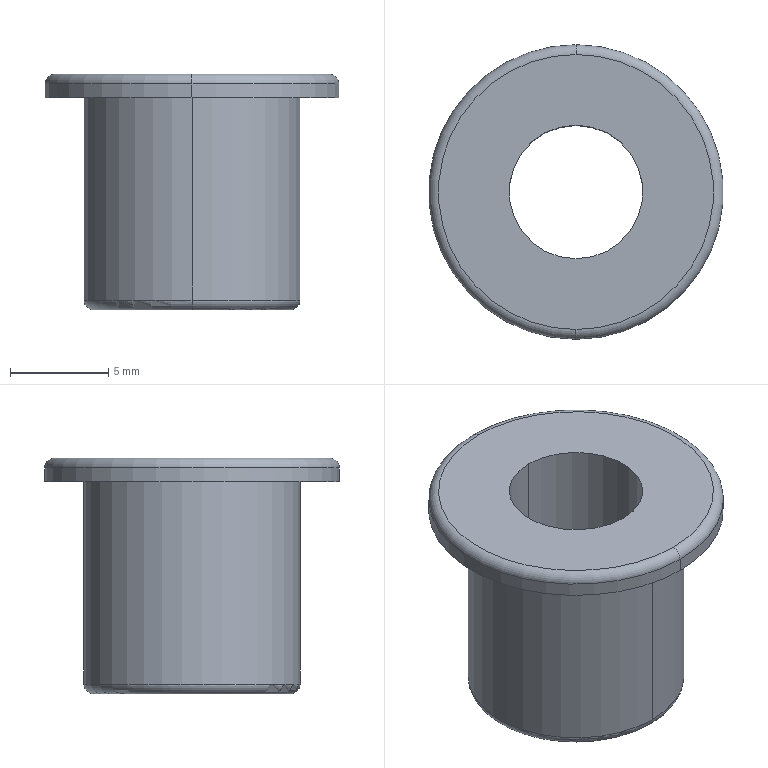Part | SolidWorks | features BaseBody 1 | 1 solid | 13 faces | box 15 x 15 x 12 mm | volume 798.307 mm3 | cylinder 6 | torus 4 | plane 3 | commonest cylinder face diameters 6.8 x2 11 x2 15 x2
STEP:
#1=CARTESIAN_POINT('',(205.5,-189.25,270.7));
#2=VERTEX_POINT('',#1);
#3=CARTESIAN_POINT('',(205.5,-204.25,270.7));
#4=VERTEX_POINT('',#3);
#5=CARTESIAN_POINT('',(205.5,-196.75,270.7));
#6=DIRECTION('',(0.,0.,1.));
#7=DIRECTION('',(0.,-1.,0.));
#8=AXIS2_PLACEMENT_3D('',#5,#6,#7);
#9=CIRCLE('',#8,7.5);
#10=EDGE_CURVE('',#2,#4,#9,.T.);
#11=ORIENTED_EDGE('',*,*,#10,.T.);
#12=CARTESIAN_POINT('',(205.5,-204.25,271.4));
#13=VERTEX_POINT('',#12);
#14=CARTESIAN_POINT('',(205.5,-204.25,270.7));
#15=DIRECTION('',(0.,0.,1.));
#16=VECTOR('',#15,1000.);
#17=LINE('',#14,#16);
#18=EDGE_CURVE('',#4,#13,#17,.T.);
#19=ORIENTED_EDGE('',*,*,#18,.T.);
#20=CARTESIAN_POINT('',(205.5,-189.25,271.4));
#21=VERTEX_POINT('',#20);
#22=CARTESIAN_POINT('',(205.5,-196.75,271.4));
#23=DIRECTION('',(0.,0.,-1.));
#24=DIRECTION('',(0.,-1.,0.));
#25=AXIS2_PLACEMENT_3D('',#22,#23,#24);
#26=CIRCLE('',#25,7.5);
#27=EDGE_CURVE('',#13,#21,#26,.T.);
#28=ORIENTED_EDGE('',*,*,#27,.T.);
#29=CARTESIAN_POINT('',(205.5,-189.25,270.7));
#30=DIRECTION('',(0.,0.,1.));
#31=VECTOR('',#30,1000.);
#32=LINE('',#29,#31);
#33=EDGE_CURVE('',#2,#21,#32,.T.);
#34=ORIENTED_EDGE('',*,*,#33,.F.);
#35=EDGE_LOOP('',(#11,#19,#28,#34));
#36=FACE_OUTER_BOUND('',#35,.T.);
#37=CARTESIAN_POINT('',(205.5,-196.75,270.7));
#38=DIRECTION('',(0.,0.,1.));
#39=DIRECTION('',(0.,1.,0.));
#40=AXIS2_PLACEMENT_3D('',#37,#38,#39);
#41=CYLINDRICAL_SURFACE('',#40,7.5);
#42=ADVANCED_FACE('',(#36),#41,.T.);
#43=CARTESIAN_POINT('',(205.5,-193.35,259.9));
#44=VERTEX_POINT('',#43);
#45=CARTESIAN_POINT('',(205.5,-200.15,259.9));
#46=VERTEX_POINT('',#45);
#47=CARTESIAN_POINT('',(205.5,-196.75,259.9));
#48=DIRECTION('',(0.,0.,-1.));
#49=DIRECTION('',(0.,-1.,0.));
#50=AXIS2_PLACEMENT_3D('',#47,#48,#49);
#51=CIRCLE('',#50,3.4);
#52=EDGE_CURVE('',#44,#46,#51,.T.);
#53=ORIENTED_EDGE('',*,*,#52,.T.);
#54=CARTESIAN_POINT('',(205.5,-200.15,271.9));
#55=VERTEX_POINT('',#54);
#56=CARTESIAN_POINT('',(205.5,-200.15,259.9));
#57=DIRECTION('',(0.,0.,1.));
#58=VECTOR('',#57,1000.);
#59=LINE('',#56,#58);
#60=EDGE_CURVE('',#46,#55,#59,.T.);
#61=ORIENTED_EDGE('',*,*,#60,.T.);
#62=CARTESIAN_POINT('',(205.5,-193.35,271.9));
#63=VERTEX_POINT('',#62);
#64=CARTESIAN_POINT('',(205.5,-196.75,271.9));
#65=DIRECTION('',(0.,0.,-1.));
#66=DIRECTION('',(0.,-1.,0.));
#67=AXIS2_PLACEMENT_3D('',#64,#65,#66);
#68=CIRCLE('',#67,3.4);
#69=EDGE_CURVE('',#63,#55,#68,.T.);
#70=ORIENTED_EDGE('',*,*,#69,.F.);
#71=CARTESIAN_POINT('',(205.5,-193.35,259.9));
#72=DIRECTION('',(0.,0.,1.));
#73=VECTOR('',#72,1000.);
#74=LINE('',#71,#73);
#75=EDGE_CURVE('',#44,#63,#74,.T.);
#76=ORIENTED_EDGE('',*,*,#75,.F.);
#77=EDGE_LOOP('',(#53,#61,#70,#76));
#78=FACE_OUTER_BOUND('',#77,.T.);
#79=CARTESIAN_POINT('',(205.5,-196.75,259.9));
#80=DIRECTION('',(0.,0.,1.));
#81=DIRECTION('',(0.,1.,0.));
#82=AXIS2_PLACEMENT_3D('',#79,#80,#81);
#83=CYLINDRICAL_SURFACE('',#82,3.4);
#84=ADVANCED_FACE('',(#78),#83,.F.);
#85=CARTESIAN_POINT('',(205.5,-191.25,260.4));
#86=VERTEX_POINT('',#85);
#87=CARTESIAN_POINT('',(205.5,-202.25,260.4));
#88=VERTEX_POINT('',#87);
#89=CARTESIAN_POINT('',(205.5,-196.75,260.4));
#90=DIRECTION('',(0.,0.,1.));
#91=DIRECTION('',(0.,-1.,0.));
#92=AXIS2_PLACEMENT_3D('',#89,#90,#91);
#93=CIRCLE('',#92,5.5);
#94=EDGE_CURVE('',#86,#88,#93,.T.);
#95=ORIENTED_EDGE('',*,*,#94,.T.);
#96=CARTESIAN_POINT('',(205.5,-202.25,270.7));
#97=VERTEX_POINT('',#96);
#98=CARTESIAN_POINT('',(205.5,-202.25,260.4));
#99=DIRECTION('',(0.,0.,1.));
#100=VECTOR('',#99,1000.);
#101=LINE('',#98,#100);
#102=EDGE_CURVE('',#88,#97,#101,.T.);
#103=ORIENTED_EDGE('',*,*,#102,.T.);
#104=CARTESIAN_POINT('',(205.5,-191.25,270.7));
#105=VERTEX_POINT('',#104);
#106=CARTESIAN_POINT('',(205.5,-196.75,270.7));
#107=DIRECTION('',(0.,0.,1.));
#108=DIRECTION('',(0.,-1.,0.));
#109=AXIS2_PLACEMENT_3D('',#106,#107,#108);
#110=CIRCLE('',#109,5.5);
#111=EDGE_CURVE('',#105,#97,#110,.T.);
#112=ORIENTED_EDGE('',*,*,#111,.F.);
#113=CARTESIAN_POINT('',(205.5,-191.25,260.4));
#114=DIRECTION('',(0.,0.,1.));
#115=VECTOR('',#114,1000.);
#116=LINE('',#113,#115);
#117=EDGE_CURVE('',#86,#105,#116,.T.);
#118=ORIENTED_EDGE('',*,*,#117,.F.);
#119=EDGE_LOOP('',(#95,#103,#112,#118));
#120=FACE_OUTER_BOUND('',#119,.T.);
#121=CARTESIAN_POINT('',(205.5,-196.75,260.4));
#122=DIRECTION('',(0.,0.,1.));
#123=DIRECTION('',(0.,1.,0.));
#124=AXIS2_PLACEMENT_3D('',#121,#122,#123);
#125=CYLINDRICAL_SURFACE('',#124,5.5);
#126=ADVANCED_FACE('',(#120),#125,.T.);
#127=ORIENTED_EDGE('',*,*,#27,.F.);
#128=CARTESIAN_POINT('',(205.5,-203.75,271.9));
#129=VERTEX_POINT('',#128);
#130=CARTESIAN_POINT('',(205.5,-203.75,271.4));
#131=DIRECTION('',(-1.,0.,0.));
#132=DIRECTION('',(0.,-1.,0.));
#133=AXIS2_PLACEMENT_3D('',#130,#131,#132);
#134=CIRCLE('',#133,0.5);
#135=EDGE_CURVE('',#13,#129,#134,.T.);
#136=ORIENTED_EDGE('',*,*,#135,.T.);
#137=CARTESIAN_POINT('',(205.5,-189.75,271.9));
#138=VERTEX_POINT('',#137);
#139=CARTESIAN_POINT('',(205.5,-196.75,271.9));
#140=DIRECTION('',(0.,0.,1.));
#141=DIRECTION('',(0.,-1.,0.));
#142=AXIS2_PLACEMENT_3D('',#139,#140,#141);
#143=CIRCLE('',#142,7.);
#144=EDGE_CURVE('',#138,#129,#143,.T.);
#145=ORIENTED_EDGE('',*,*,#144,.F.);
#146=CARTESIAN_POINT('',(205.5,-189.75,271.4));
#147=DIRECTION('',(1.,0.,0.));
#148=DIRECTION('',(0.,1.,0.));
#149=AXIS2_PLACEMENT_3D('',#146,#147,#148);
#150=CIRCLE('',#149,0.5);
#151=EDGE_CURVE('',#21,#138,#150,.T.);
#152=ORIENTED_EDGE('',*,*,#151,.F.);
#153=EDGE_LOOP('',(#127,#136,#145,#152));
#154=FACE_OUTER_BOUND('',#153,.T.);
#155=CARTESIAN_POINT('',(205.5,-196.75,271.4));
#156=DIRECTION('',(0.,0.,1.));
#157=DIRECTION('',(0.,1.,0.));
#158=AXIS2_PLACEMENT_3D('',#155,#156,#157);
#159=TOROIDAL_SURFACE('',#158,7.,0.5);
#160=ADVANCED_FACE('',(#154),#159,.T.);
#161=CARTESIAN_POINT('',(205.5,-201.75,259.9));
#162=VERTEX_POINT('',#161);
#163=CARTESIAN_POINT('',(205.5,-191.75,259.9));
#164=VERTEX_POINT('',#163);
#165=CARTESIAN_POINT('',(205.5,-196.75,259.9));
#166=DIRECTION('',(0.,0.,-1.));
#167=DIRECTION('',(0.,-1.,0.));
#168=AXIS2_PLACEMENT_3D('',#165,#166,#167);
#169=CIRCLE('',#168,5.);
#170=EDGE_CURVE('',#162,#164,#169,.T.);
#171=ORIENTED_EDGE('',*,*,#170,.F.);
#172=CARTESIAN_POINT('',(205.5,-201.75,260.4));
#173=DIRECTION('',(-1.,0.,0.));
#174=DIRECTION('',(0.,-1.,0.));
#175=AXIS2_PLACEMENT_3D('',#172,#173,#174);
#176=CIRCLE('',#175,0.5);
#177=EDGE_CURVE('',#162,#88,#176,.T.);
#178=ORIENTED_EDGE('',*,*,#177,.T.);
#179=ORIENTED_EDGE('',*,*,#94,.F.);
#180=CARTESIAN_POINT('',(205.5,-191.75,260.4));
#181=DIRECTION('',(1.,0.,0.));
#182=DIRECTION('',(0.,1.,0.));
#183=AXIS2_PLACEMENT_3D('',#180,#181,#182);
#184=CIRCLE('',#183,0.5);
#185=EDGE_CURVE('',#164,#86,#184,.T.);
#186=ORIENTED_EDGE('',*,*,#185,.F.);
#187=EDGE_LOOP('',(#171,#178,#179,#186));
#188=FACE_OUTER_BOUND('',#187,.T.);
#189=CARTESIAN_POINT('',(205.5,-196.75,260.4));
#190=DIRECTION('',(0.,0.,1.));
#191=DIRECTION('',(0.,1.,0.));
#192=AXIS2_PLACEMENT_3D('',#189,#190,#191);
#193=TOROIDAL_SURFACE('',#192,5.,0.5);
#194=ADVANCED_FACE('',(#188),#193,.T.);
#195=ORIENTED_EDGE('',*,*,#177,.F.);
#196=CARTESIAN_POINT('',(205.5,-196.75,259.9));
#197=DIRECTION('',(0.,0.,-1.));
#198=DIRECTION('',(0.,-1.,0.));
#199=AXIS2_PLACEMENT_3D('',#196,#197,#198);
#200=CIRCLE('',#199,5.);
#201=EDGE_CURVE('',#164,#162,#200,.T.);
#202=ORIENTED_EDGE('',*,*,#201,.F.);
#203=ORIENTED_EDGE('',*,*,#185,.T.);
#204=CARTESIAN_POINT('',(205.5,-196.75,260.4));
#205=DIRECTION('',(0.,0.,1.));
#206=DIRECTION('',(0.,-1.,0.));
#207=AXIS2_PLACEMENT_3D('',#204,#205,#206);
#208=CIRCLE('',#207,5.5);
#209=EDGE_CURVE('',#88,#86,#208,.T.);
#210=ORIENTED_EDGE('',*,*,#209,.F.);
#211=EDGE_LOOP('',(#195,#202,#203,#210));
#212=FACE_OUTER_BOUND('',#211,.T.);
#213=CARTESIAN_POINT('',(205.5,-196.75,260.4));
#214=DIRECTION('',(0.,0.,1.));
#215=DIRECTION('',(0.,1.,0.));
#216=AXIS2_PLACEMENT_3D('',#213,#214,#215);
#217=TOROIDAL_SURFACE('',#216,5.,0.5);
#218=ADVANCED_FACE('',(#212),#217,.T.);
#219=ORIENTED_EDGE('',*,*,#135,.F.);
#220=CARTESIAN_POINT('',(205.5,-196.75,271.4));
#221=DIRECTION('',(0.,0.,-1.));
#222=DIRECTION('',(0.,-1.,0.));
#223=AXIS2_PLACEMENT_3D('',#220,#221,#222);
#224=CIRCLE('',#223,7.5);
#225=EDGE_CURVE('',#21,#13,#224,.T.);
#226=ORIENTED_EDGE('',*,*,#225,.F.);
#227=ORIENTED_EDGE('',*,*,#151,.T.);
#228=CARTESIAN_POINT('',(205.5,-196.75,271.9));
#229=DIRECTION('',(0.,0.,1.));
#230=DIRECTION('',(0.,-1.,0.));
#231=AXIS2_PLACEMENT_3D('',#228,#229,#230);
#232=CIRCLE('',#231,7.);
#233=EDGE_CURVE('',#129,#138,#232,.T.);
#234=ORIENTED_EDGE('',*,*,#233,.F.);
#235=EDGE_LOOP('',(#219,#226,#227,#234));
#236=FACE_OUTER_BOUND('',#235,.T.);
#237=CARTESIAN_POINT('',(205.5,-196.75,271.4));
#238=DIRECTION('',(0.,0.,1.));
#239=DIRECTION('',(0.,1.,0.));
#240=AXIS2_PLACEMENT_3D('',#237,#238,#239);
#241=TOROIDAL_SURFACE('',#240,7.,0.5);
#242=ADVANCED_FACE('',(#236),#241,.T.);
#243=ORIENTED_EDGE('',*,*,#52,.F.);
#244=CARTESIAN_POINT('',(205.5,-196.75,259.9));
#245=DIRECTION('',(0.,0.,-1.));
#246=DIRECTION('',(0.,-1.,0.));
#247=AXIS2_PLACEMENT_3D('',#244,#245,#246);
#248=CIRCLE('',#247,3.4);
#249=EDGE_CURVE('',#46,#44,#248,.T.);
#250=ORIENTED_EDGE('',*,*,#249,.F.);
#251=EDGE_LOOP('',(#243,#250));
#252=FACE_BOUND('',#251,.T.);
#253=ORIENTED_EDGE('',*,*,#201,.T.);
#254=ORIENTED_EDGE('',*,*,#170,.T.);
#255=EDGE_LOOP('',(#253,#254));
#256=FACE_OUTER_BOUND('',#255,.T.);
#257=CARTESIAN_POINT('',(205.5,-195.276,259.9));
#258=DIRECTION('',(0.,0.,-1.));
#259=DIRECTION('',(-1.,0.,0.));
#260=AXIS2_PLACEMENT_3D('',#257,#258,#259);
#261=PLANE('',#260);
#262=ADVANCED_FACE('',(#252,#256),#261,.T.);
#263=ORIENTED_EDGE('',*,*,#102,.F.);
#264=ORIENTED_EDGE('',*,*,#209,.T.);
#265=ORIENTED_EDGE('',*,*,#117,.T.);
#266=CARTESIAN_POINT('',(205.5,-196.75,270.7));
#267=DIRECTION('',(0.,0.,1.));
#268=DIRECTION('',(0.,-1.,0.));
#269=AXIS2_PLACEMENT_3D('',#266,#267,#268);
#270=CIRCLE('',#269,5.5);
#271=EDGE_CURVE('',#97,#105,#270,.T.);
#272=ORIENTED_EDGE('',*,*,#271,.F.);
#273=EDGE_LOOP('',(#263,#264,#265,#272));
#274=FACE_OUTER_BOUND('',#273,.T.);
#275=CARTESIAN_POINT('',(205.5,-196.75,260.4));
#276=DIRECTION('',(0.,0.,1.));
#277=DIRECTION('',(0.,1.,0.));
#278=AXIS2_PLACEMENT_3D('',#275,#276,#277);
#279=CYLINDRICAL_SURFACE('',#278,5.5);
#280=ADVANCED_FACE('',(#274),#279,.T.);
#281=ORIENTED_EDGE('',*,*,#60,.F.);
#282=ORIENTED_EDGE('',*,*,#249,.T.);
#283=ORIENTED_EDGE('',*,*,#75,.T.);
#284=CARTESIAN_POINT('',(205.5,-196.75,271.9));
#285=DIRECTION('',(0.,0.,-1.));
#286=DIRECTION('',(0.,-1.,0.));
#287=AXIS2_PLACEMENT_3D('',#284,#285,#286);
#288=CIRCLE('',#287,3.4);
#289=EDGE_CURVE('',#55,#63,#288,.T.);
#290=ORIENTED_EDGE('',*,*,#289,.F.);
#291=EDGE_LOOP('',(#281,#282,#283,#290));
#292=FACE_OUTER_BOUND('',#291,.T.);
#293=CARTESIAN_POINT('',(205.5,-196.75,259.9));
#294=DIRECTION('',(0.,0.,1.));
#295=DIRECTION('',(0.,1.,0.));
#296=AXIS2_PLACEMENT_3D('',#293,#294,#295);
#297=CYLINDRICAL_SURFACE('',#296,3.4);
#298=ADVANCED_FACE('',(#292),#297,.F.);
#299=ORIENTED_EDGE('',*,*,#111,.T.);
#300=ORIENTED_EDGE('',*,*,#271,.T.);
#301=EDGE_LOOP('',(#299,#300));
#302=FACE_BOUND('',#301,.T.);
#303=ORIENTED_EDGE('',*,*,#10,.F.);
#304=CARTESIAN_POINT('',(205.5,-196.75,270.7));
#305=DIRECTION('',(0.,0.,1.));
#306=DIRECTION('',(0.,-1.,0.));
#307=AXIS2_PLACEMENT_3D('',#304,#305,#306);
#308=CIRCLE('',#307,7.5);
#309=EDGE_CURVE('',#4,#2,#308,.T.);
#310=ORIENTED_EDGE('',*,*,#309,.F.);
#311=EDGE_LOOP('',(#303,#310));
#312=FACE_OUTER_BOUND('',#311,.T.);
#313=CARTESIAN_POINT('',(205.5,-194.74,270.7));
#314=DIRECTION('',(0.,0.,-1.));
#315=DIRECTION('',(-1.,0.,0.));
#316=AXIS2_PLACEMENT_3D('',#313,#314,#315);
#317=PLANE('',#316);
#318=ADVANCED_FACE('',(#302,#312),#317,.T.);
#319=ORIENTED_EDGE('',*,*,#18,.F.);
#320=ORIENTED_EDGE('',*,*,#309,.T.);
#321=ORIENTED_EDGE('',*,*,#33,.T.);
#322=ORIENTED_EDGE('',*,*,#225,.T.);
#323=EDGE_LOOP('',(#319,#320,#321,#322));
#324=FACE_OUTER_BOUND('',#323,.T.);
#325=CARTESIAN_POINT('',(205.5,-196.75,270.7));
#326=DIRECTION('',(0.,0.,1.));
#327=DIRECTION('',(0.,1.,0.));
#328=AXIS2_PLACEMENT_3D('',#325,#326,#327);
#329=CYLINDRICAL_SURFACE('',#328,7.5);
#330=ADVANCED_FACE('',(#324),#329,.T.);
#331=ORIENTED_EDGE('',*,*,#69,.T.);
#332=ORIENTED_EDGE('',*,*,#289,.T.);
#333=EDGE_LOOP('',(#331,#332));
#334=FACE_BOUND('',#333,.T.);
#335=ORIENTED_EDGE('',*,*,#144,.T.);
#336=ORIENTED_EDGE('',*,*,#233,.T.);
#337=EDGE_LOOP('',(#335,#336));
#338=FACE_OUTER_BOUND('',#337,.T.);
#339=CARTESIAN_POINT('',(205.5,-194.74,271.9));
#340=DIRECTION('',(0.,0.,1.));
#341=DIRECTION('',(1.,0.,0.));
#342=AXIS2_PLACEMENT_3D('',#339,#340,#341);
#343=PLANE('',#342);
#344=ADVANCED_FACE('',(#334,#338),#343,.T.);
#345=CLOSED_SHELL('',(#42,#84,#126,#160,#194,#218,#242,#262,#280,#298,#318,#330,#344));
#346=MANIFOLD_SOLID_BREP('',#345);
#347=CARTESIAN_POINT('',(0.,0.,0.));
#348=DIRECTION('',(0.,0.,1.));
#349=DIRECTION('',(1.,0.,0.));
#350=AXIS2_PLACEMENT_3D('',#347,#348,#349);
#351=(LENGTH_UNIT()NAMED_UNIT(*)SI_UNIT(.MILLI.,.METRE.));
#352=UNCERTAINTY_MEASURE_WITH_UNIT(LENGTH_MEASURE(0.00001),#351,'','');
#353=(NAMED_UNIT(*)PLANE_ANGLE_UNIT()SI_UNIT($,.RADIAN.));
#354=(NAMED_UNIT(*)SI_UNIT($,.STERADIAN.)SOLID_ANGLE_UNIT());
#355=(GEOMETRIC_REPRESENTATION_CONTEXT(3)GLOBAL_UNCERTAINTY_ASSIGNED_CONTEXT((#352))GLOBAL_UNIT_ASSIGNED_CONTEXT((#351,#353,#354))REPRESENTATION_CONTEXT('',''));
#356=ADVANCED_BREP_SHAPE_REPRESENTATION('',(#346,#350),#355);